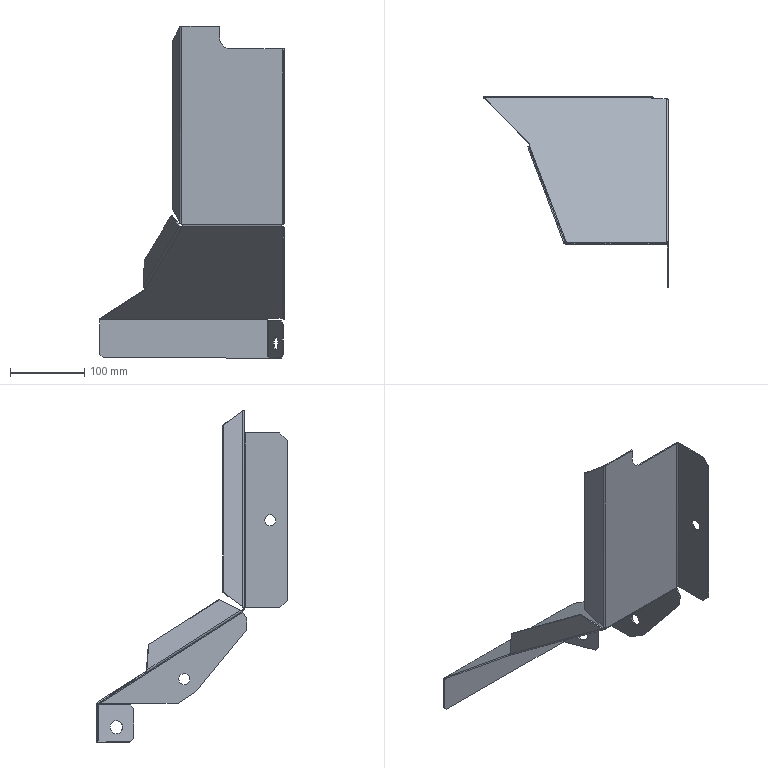Part | SolidWorks | features SM3dBend 7, FlatPattern 1, SMBaseFlange 1, SheetMetal 1 | 1 solid | 96 faces | box 249.839 x 257.358 x 448.59 mm | volume 199881 mm3 | plane 55 | cylinder 28 | spline 13 | commonest cylinder face diameters 3 x7 5 x7 6.2 x7 15 x4 18 x2 30 x1